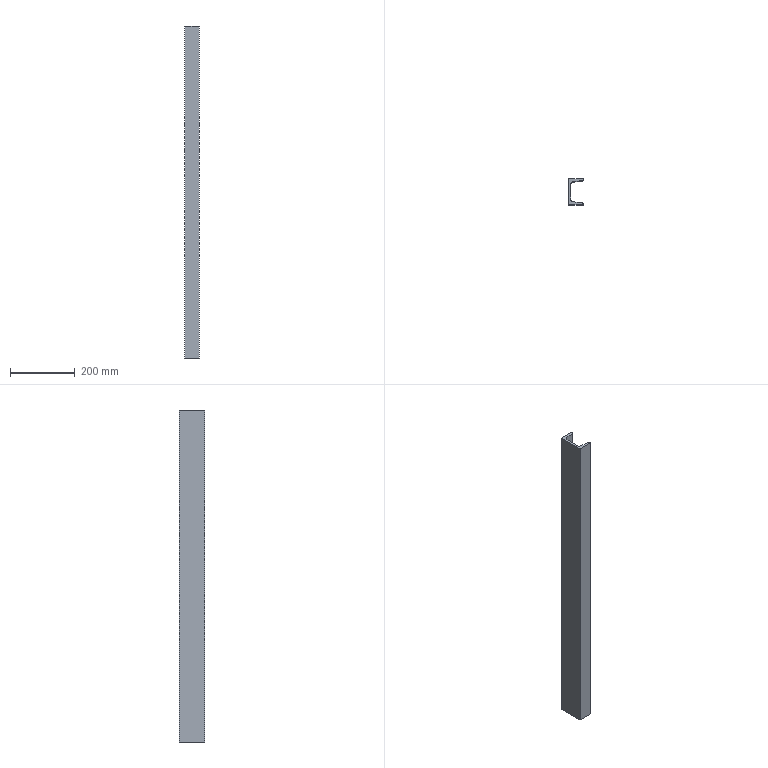Part | SolidWorks | features Extrusion 1 | 1 solid | 14 faces | box 45 x 80 x 1022 mm | volume 1109758 mm3 | plane 10 | cylinder 4 | commonest cylinder face diameters 8 x2 16 x2
STEP:
#1=CARTESIAN_POINT('',(-3.443,-5.322,0.));
#2=VERTEX_POINT('',#1);
#3=CARTESIAN_POINT('',(0.,-1.361,0.));
#4=VERTEX_POINT('',#3);
#5=CARTESIAN_POINT('',(-4.,-1.361,0.));
#6=DIRECTION('',(0.,0.,1.));
#7=DIRECTION('',(1.,0.,0.));
#8=AXIS2_PLACEMENT_3D('',#5,#6,#7);
#9=CIRCLE('',#8,4.);
#10=EDGE_CURVE('',#2,#4,#9,.T.);
#11=ORIENTED_EDGE('',*,*,#10,.T.);
#12=CARTESIAN_POINT('',(0.,-1.361,1022.));
#13=VERTEX_POINT('',#12);
#14=CARTESIAN_POINT('',(0.,-1.361,1022.));
#15=DIRECTION('',(0.,0.,-1.));
#16=VECTOR('',#15,1000.);
#17=LINE('',#14,#16);
#18=EDGE_CURVE('',#13,#4,#17,.T.);
#19=ORIENTED_EDGE('',*,*,#18,.F.);
#20=CARTESIAN_POINT('',(-3.443,-5.322,1022.));
#21=VERTEX_POINT('',#20);
#22=CARTESIAN_POINT('',(-4.,-1.361,1022.));
#23=DIRECTION('',(0.,0.,1.));
#24=DIRECTION('',(1.,0.,0.));
#25=AXIS2_PLACEMENT_3D('',#22,#23,#24);
#26=CIRCLE('',#25,4.);
#27=EDGE_CURVE('',#21,#13,#26,.T.);
#28=ORIENTED_EDGE('',*,*,#27,.F.);
#29=CARTESIAN_POINT('',(-3.443,-5.322,1022.));
#30=DIRECTION('',(0.,0.,-1.));
#31=VECTOR('',#30,1000.);
#32=LINE('',#29,#31);
#33=EDGE_CURVE('',#21,#2,#32,.T.);
#34=ORIENTED_EDGE('',*,*,#33,.T.);
#35=EDGE_LOOP('',(#11,#19,#28,#34));
#36=FACE_OUTER_BOUND('',#35,.T.);
#37=CARTESIAN_POINT('',(-4.,-1.361,1022.));
#38=DIRECTION('',(0.,0.,-1.));
#39=DIRECTION('',(-1.,0.,0.));
#40=AXIS2_PLACEMENT_3D('',#37,#38,#39);
#41=CYLINDRICAL_SURFACE('',#40,4.);
#42=ADVANCED_FACE('',(#36),#41,.T.);
#43=CARTESIAN_POINT('',(0.,0.,0.));
#44=VERTEX_POINT('',#43);
#45=CARTESIAN_POINT('',(0.,-1.361,0.));
#46=DIRECTION('',(0.,1.,0.));
#47=VECTOR('',#46,1000.);
#48=LINE('',#45,#47);
#49=EDGE_CURVE('',#4,#44,#48,.T.);
#50=ORIENTED_EDGE('',*,*,#49,.T.);
#51=CARTESIAN_POINT('',(0.,0.,1022.));
#52=VERTEX_POINT('',#51);
#53=CARTESIAN_POINT('',(0.,0.,1022.));
#54=DIRECTION('',(0.,0.,-1.));
#55=VECTOR('',#54,1000.);
#56=LINE('',#53,#55);
#57=EDGE_CURVE('',#52,#44,#56,.T.);
#58=ORIENTED_EDGE('',*,*,#57,.F.);
#59=CARTESIAN_POINT('',(0.,-1.361,1022.));
#60=DIRECTION('',(0.,1.,0.));
#61=VECTOR('',#60,1000.);
#62=LINE('',#59,#61);
#63=EDGE_CURVE('',#13,#52,#62,.T.);
#64=ORIENTED_EDGE('',*,*,#63,.F.);
#65=ORIENTED_EDGE('',*,*,#18,.T.);
#66=EDGE_LOOP('',(#50,#58,#64,#65));
#67=FACE_OUTER_BOUND('',#66,.T.);
#68=CARTESIAN_POINT('',(0.,-1.361,1022.));
#69=DIRECTION('',(-1.,0.,0.));
#70=DIRECTION('',(0.,0.,1.));
#71=AXIS2_PLACEMENT_3D('',#68,#69,#70);
#72=PLANE('',#71);
#73=ADVANCED_FACE('',(#67),#72,.F.);
#74=CARTESIAN_POINT('',(-45.,0.,0.));
#75=VERTEX_POINT('',#74);
#76=CARTESIAN_POINT('',(0.,0.,0.));
#77=DIRECTION('',(-1.,0.,0.));
#78=VECTOR('',#77,1000.);
#79=LINE('',#76,#78);
#80=EDGE_CURVE('',#44,#75,#79,.T.);
#81=ORIENTED_EDGE('',*,*,#80,.T.);
#82=CARTESIAN_POINT('',(-45.,0.,1022.));
#83=VERTEX_POINT('',#82);
#84=CARTESIAN_POINT('',(-45.,0.,1022.));
#85=DIRECTION('',(0.,0.,-1.));
#86=VECTOR('',#85,1000.);
#87=LINE('',#84,#86);
#88=EDGE_CURVE('',#83,#75,#87,.T.);
#89=ORIENTED_EDGE('',*,*,#88,.F.);
#90=CARTESIAN_POINT('',(0.,0.,1022.));
#91=DIRECTION('',(-1.,0.,0.));
#92=VECTOR('',#91,1000.);
#93=LINE('',#90,#92);
#94=EDGE_CURVE('',#52,#83,#93,.T.);
#95=ORIENTED_EDGE('',*,*,#94,.F.);
#96=ORIENTED_EDGE('',*,*,#57,.T.);
#97=EDGE_LOOP('',(#81,#89,#95,#96));
#98=FACE_OUTER_BOUND('',#97,.T.);
#99=CARTESIAN_POINT('',(0.,0.,1022.));
#100=DIRECTION('',(0.,-1.,0.));
#101=DIRECTION('',(1.,0.,0.));
#102=AXIS2_PLACEMENT_3D('',#99,#100,#101);
#103=PLANE('',#102);
#104=ADVANCED_FACE('',(#98),#103,.F.);
#105=CARTESIAN_POINT('',(-45.,-80.,0.));
#106=VERTEX_POINT('',#105);
#107=CARTESIAN_POINT('',(-45.,0.,0.));
#108=DIRECTION('',(0.,-1.,0.));
#109=VECTOR('',#108,1000.);
#110=LINE('',#107,#109);
#111=EDGE_CURVE('',#75,#106,#110,.T.);
#112=ORIENTED_EDGE('',*,*,#111,.T.);
#113=CARTESIAN_POINT('',(-45.,-80.,1022.));
#114=VERTEX_POINT('',#113);
#115=CARTESIAN_POINT('',(-45.,-80.,1022.));
#116=DIRECTION('',(0.,0.,-1.));
#117=VECTOR('',#116,1000.);
#118=LINE('',#115,#117);
#119=EDGE_CURVE('',#114,#106,#118,.T.);
#120=ORIENTED_EDGE('',*,*,#119,.F.);
#121=CARTESIAN_POINT('',(-45.,0.,1022.));
#122=DIRECTION('',(0.,-1.,0.));
#123=VECTOR('',#122,1000.);
#124=LINE('',#121,#123);
#125=EDGE_CURVE('',#83,#114,#124,.T.);
#126=ORIENTED_EDGE('',*,*,#125,.F.);
#127=ORIENTED_EDGE('',*,*,#88,.T.);
#128=EDGE_LOOP('',(#112,#120,#126,#127));
#129=FACE_OUTER_BOUND('',#128,.T.);
#130=CARTESIAN_POINT('',(-45.,0.,1022.));
#131=DIRECTION('',(1.,0.,0.));
#132=DIRECTION('',(0.,1.,0.));
#133=AXIS2_PLACEMENT_3D('',#130,#131,#132);
#134=PLANE('',#133);
#135=ADVANCED_FACE('',(#129),#134,.F.);
#136=CARTESIAN_POINT('',(0.,-80.,0.));
#137=VERTEX_POINT('',#136);
#138=CARTESIAN_POINT('',(-45.,-80.,0.));
#139=DIRECTION('',(1.,0.,0.));
#140=VECTOR('',#139,1000.);
#141=LINE('',#138,#140);
#142=EDGE_CURVE('',#106,#137,#141,.T.);
#143=ORIENTED_EDGE('',*,*,#142,.T.);
#144=CARTESIAN_POINT('',(0.,-80.,1022.));
#145=VERTEX_POINT('',#144);
#146=CARTESIAN_POINT('',(0.,-80.,1022.));
#147=DIRECTION('',(0.,0.,-1.));
#148=VECTOR('',#147,1000.);
#149=LINE('',#146,#148);
#150=EDGE_CURVE('',#145,#137,#149,.T.);
#151=ORIENTED_EDGE('',*,*,#150,.F.);
#152=CARTESIAN_POINT('',(-45.,-80.,1022.));
#153=DIRECTION('',(1.,0.,0.));
#154=VECTOR('',#153,1000.);
#155=LINE('',#152,#154);
#156=EDGE_CURVE('',#114,#145,#155,.T.);
#157=ORIENTED_EDGE('',*,*,#156,.F.);
#158=ORIENTED_EDGE('',*,*,#119,.T.);
#159=EDGE_LOOP('',(#143,#151,#157,#158));
#160=FACE_OUTER_BOUND('',#159,.T.);
#161=CARTESIAN_POINT('',(-45.,-80.,1022.));
#162=DIRECTION('',(0.,1.,0.));
#163=DIRECTION('',(-1.,0.,0.));
#164=AXIS2_PLACEMENT_3D('',#161,#162,#163);
#165=PLANE('',#164);
#166=ADVANCED_FACE('',(#160),#165,.F.);
#167=CARTESIAN_POINT('',(0.,-78.639,0.));
#168=VERTEX_POINT('',#167);
#169=CARTESIAN_POINT('',(0.,-80.,0.));
#170=DIRECTION('',(0.,1.,0.));
#171=VECTOR('',#170,1000.);
#172=LINE('',#169,#171);
#173=EDGE_CURVE('',#137,#168,#172,.T.);
#174=ORIENTED_EDGE('',*,*,#173,.T.);
#175=CARTESIAN_POINT('',(0.,-78.639,1022.));
#176=VERTEX_POINT('',#175);
#177=CARTESIAN_POINT('',(0.,-78.639,1022.));
#178=DIRECTION('',(0.,0.,-1.));
#179=VECTOR('',#178,1000.);
#180=LINE('',#177,#179);
#181=EDGE_CURVE('',#176,#168,#180,.T.);
#182=ORIENTED_EDGE('',*,*,#181,.F.);
#183=CARTESIAN_POINT('',(0.,-80.,1022.));
#184=DIRECTION('',(0.,1.,0.));
#185=VECTOR('',#184,1000.);
#186=LINE('',#183,#185);
#187=EDGE_CURVE('',#145,#176,#186,.T.);
#188=ORIENTED_EDGE('',*,*,#187,.F.);
#189=ORIENTED_EDGE('',*,*,#150,.T.);
#190=EDGE_LOOP('',(#174,#182,#188,#189));
#191=FACE_OUTER_BOUND('',#190,.T.);
#192=CARTESIAN_POINT('',(0.,-80.,1022.));
#193=DIRECTION('',(-1.,0.,0.));
#194=DIRECTION('',(0.,0.,1.));
#195=AXIS2_PLACEMENT_3D('',#192,#193,#194);
#196=PLANE('',#195);
#197=ADVANCED_FACE('',(#191),#196,.F.);
#198=CARTESIAN_POINT('',(-3.443,-74.678,0.));
#199=VERTEX_POINT('',#198);
#200=CARTESIAN_POINT('',(-4.,-78.639,0.));
#201=DIRECTION('',(0.,0.,1.));
#202=DIRECTION('',(1.,0.,0.));
#203=AXIS2_PLACEMENT_3D('',#200,#201,#202);
#204=CIRCLE('',#203,4.);
#205=EDGE_CURVE('',#168,#199,#204,.T.);
#206=ORIENTED_EDGE('',*,*,#205,.T.);
#207=CARTESIAN_POINT('',(-3.443,-74.678,1022.));
#208=VERTEX_POINT('',#207);
#209=CARTESIAN_POINT('',(-3.443,-74.678,1022.));
#210=DIRECTION('',(0.,0.,-1.));
#211=VECTOR('',#210,1000.);
#212=LINE('',#209,#211);
#213=EDGE_CURVE('',#208,#199,#212,.T.);
#214=ORIENTED_EDGE('',*,*,#213,.F.);
#215=CARTESIAN_POINT('',(-4.,-78.639,1022.));
#216=DIRECTION('',(0.,0.,1.));
#217=DIRECTION('',(1.,0.,0.));
#218=AXIS2_PLACEMENT_3D('',#215,#216,#217);
#219=CIRCLE('',#218,4.);
#220=EDGE_CURVE('',#176,#208,#219,.T.);
#221=ORIENTED_EDGE('',*,*,#220,.F.);
#222=ORIENTED_EDGE('',*,*,#181,.T.);
#223=EDGE_LOOP('',(#206,#214,#221,#222));
#224=FACE_OUTER_BOUND('',#223,.T.);
#225=CARTESIAN_POINT('',(-4.,-78.639,1022.));
#226=DIRECTION('',(0.,0.,-1.));
#227=DIRECTION('',(-1.,0.,0.));
#228=AXIS2_PLACEMENT_3D('',#225,#226,#227);
#229=CYLINDRICAL_SURFACE('',#228,4.);
#230=ADVANCED_FACE('',(#224),#229,.T.);
#231=CARTESIAN_POINT('',(-32.113,-70.649,0.));
#232=VERTEX_POINT('',#231);
#233=CARTESIAN_POINT('',(-3.443,-74.678,0.));
#234=DIRECTION('',(-0.9903,0.1392,0.));
#235=VECTOR('',#234,1000.);
#236=LINE('',#233,#235);
#237=EDGE_CURVE('',#199,#232,#236,.T.);
#238=ORIENTED_EDGE('',*,*,#237,.T.);
#239=CARTESIAN_POINT('',(-32.113,-70.649,1022.));
#240=VERTEX_POINT('',#239);
#241=CARTESIAN_POINT('',(-32.113,-70.649,1022.));
#242=DIRECTION('',(0.,0.,-1.));
#243=VECTOR('',#242,1000.);
#244=LINE('',#241,#243);
#245=EDGE_CURVE('',#240,#232,#244,.T.);
#246=ORIENTED_EDGE('',*,*,#245,.F.);
#247=CARTESIAN_POINT('',(-3.443,-74.678,1022.));
#248=DIRECTION('',(-0.9903,0.1392,0.));
#249=VECTOR('',#248,1000.);
#250=LINE('',#247,#249);
#251=EDGE_CURVE('',#208,#240,#250,.T.);
#252=ORIENTED_EDGE('',*,*,#251,.F.);
#253=ORIENTED_EDGE('',*,*,#213,.T.);
#254=EDGE_LOOP('',(#238,#246,#252,#253));
#255=FACE_OUTER_BOUND('',#254,.T.);
#256=CARTESIAN_POINT('',(-3.443,-74.678,1022.));
#257=DIRECTION('',(-0.1392,-0.9903,0.));
#258=DIRECTION('',(0.9903,-0.1392,0.));
#259=AXIS2_PLACEMENT_3D('',#256,#257,#258);
#260=PLANE('',#259);
#261=ADVANCED_FACE('',(#255),#260,.F.);
#262=CARTESIAN_POINT('',(-39.,-62.727,0.));
#263=VERTEX_POINT('',#262);
#264=CARTESIAN_POINT('',(-31.,-62.727,0.));
#265=DIRECTION('',(0.,0.,-1.));
#266=DIRECTION('',(-1.,0.,0.));
#267=AXIS2_PLACEMENT_3D('',#264,#265,#266);
#268=CIRCLE('',#267,8.);
#269=EDGE_CURVE('',#232,#263,#268,.T.);
#270=ORIENTED_EDGE('',*,*,#269,.T.);
#271=CARTESIAN_POINT('',(-39.,-62.727,1022.));
#272=VERTEX_POINT('',#271);
#273=CARTESIAN_POINT('',(-39.,-62.727,1022.));
#274=DIRECTION('',(0.,0.,-1.));
#275=VECTOR('',#274,1000.);
#276=LINE('',#273,#275);
#277=EDGE_CURVE('',#272,#263,#276,.T.);
#278=ORIENTED_EDGE('',*,*,#277,.F.);
#279=CARTESIAN_POINT('',(-31.,-62.727,1022.));
#280=DIRECTION('',(0.,0.,-1.));
#281=DIRECTION('',(-1.,0.,0.));
#282=AXIS2_PLACEMENT_3D('',#279,#280,#281);
#283=CIRCLE('',#282,8.);
#284=EDGE_CURVE('',#240,#272,#283,.T.);
#285=ORIENTED_EDGE('',*,*,#284,.F.);
#286=ORIENTED_EDGE('',*,*,#245,.T.);
#287=EDGE_LOOP('',(#270,#278,#285,#286));
#288=FACE_OUTER_BOUND('',#287,.T.);
#289=CARTESIAN_POINT('',(-31.,-62.727,1022.));
#290=DIRECTION('',(0.,0.,-1.));
#291=DIRECTION('',(-1.,0.,0.));
#292=AXIS2_PLACEMENT_3D('',#289,#290,#291);
#293=CYLINDRICAL_SURFACE('',#292,8.);
#294=ADVANCED_FACE('',(#288),#293,.F.);
#295=CARTESIAN_POINT('',(-39.,-17.273,0.));
#296=VERTEX_POINT('',#295);
#297=CARTESIAN_POINT('',(-39.,-62.727,0.));
#298=DIRECTION('',(0.,1.,0.));
#299=VECTOR('',#298,1000.);
#300=LINE('',#297,#299);
#301=EDGE_CURVE('',#263,#296,#300,.T.);
#302=ORIENTED_EDGE('',*,*,#301,.T.);
#303=CARTESIAN_POINT('',(-39.,-17.273,1022.));
#304=VERTEX_POINT('',#303);
#305=CARTESIAN_POINT('',(-39.,-17.273,1022.));
#306=DIRECTION('',(0.,0.,-1.));
#307=VECTOR('',#306,1000.);
#308=LINE('',#305,#307);
#309=EDGE_CURVE('',#304,#296,#308,.T.);
#310=ORIENTED_EDGE('',*,*,#309,.F.);
#311=CARTESIAN_POINT('',(-39.,-62.727,1022.));
#312=DIRECTION('',(0.,1.,0.));
#313=VECTOR('',#312,1000.);
#314=LINE('',#311,#313);
#315=EDGE_CURVE('',#272,#304,#314,.T.);
#316=ORIENTED_EDGE('',*,*,#315,.F.);
#317=ORIENTED_EDGE('',*,*,#277,.T.);
#318=EDGE_LOOP('',(#302,#310,#316,#317));
#319=FACE_OUTER_BOUND('',#318,.T.);
#320=CARTESIAN_POINT('',(-39.,-62.727,1022.));
#321=DIRECTION('',(-1.,0.,0.));
#322=DIRECTION('',(0.,0.,1.));
#323=AXIS2_PLACEMENT_3D('',#320,#321,#322);
#324=PLANE('',#323);
#325=ADVANCED_FACE('',(#319),#324,.F.);
#326=CARTESIAN_POINT('',(-32.113,-9.351,0.));
#327=VERTEX_POINT('',#326);
#328=CARTESIAN_POINT('',(-31.,-17.273,0.));
#329=DIRECTION('',(0.,0.,-1.));
#330=DIRECTION('',(-1.,0.,0.));
#331=AXIS2_PLACEMENT_3D('',#328,#329,#330);
#332=CIRCLE('',#331,8.);
#333=EDGE_CURVE('',#296,#327,#332,.T.);
#334=ORIENTED_EDGE('',*,*,#333,.T.);
#335=CARTESIAN_POINT('',(-32.113,-9.351,1022.));
#336=VERTEX_POINT('',#335);
#337=CARTESIAN_POINT('',(-32.113,-9.351,1022.));
#338=DIRECTION('',(0.,0.,-1.));
#339=VECTOR('',#338,1000.);
#340=LINE('',#337,#339);
#341=EDGE_CURVE('',#336,#327,#340,.T.);
#342=ORIENTED_EDGE('',*,*,#341,.F.);
#343=CARTESIAN_POINT('',(-31.,-17.273,1022.));
#344=DIRECTION('',(0.,0.,-1.));
#345=DIRECTION('',(-1.,0.,0.));
#346=AXIS2_PLACEMENT_3D('',#343,#344,#345);
#347=CIRCLE('',#346,8.);
#348=EDGE_CURVE('',#304,#336,#347,.T.);
#349=ORIENTED_EDGE('',*,*,#348,.F.);
#350=ORIENTED_EDGE('',*,*,#309,.T.);
#351=EDGE_LOOP('',(#334,#342,#349,#350));
#352=FACE_OUTER_BOUND('',#351,.T.);
#353=CARTESIAN_POINT('',(-31.,-17.273,1022.));
#354=DIRECTION('',(0.,0.,-1.));
#355=DIRECTION('',(-1.,0.,0.));
#356=AXIS2_PLACEMENT_3D('',#353,#354,#355);
#357=CYLINDRICAL_SURFACE('',#356,8.);
#358=ADVANCED_FACE('',(#352),#357,.F.);
#359=CARTESIAN_POINT('',(-32.113,-9.351,0.));
#360=DIRECTION('',(0.9903,0.1392,0.));
#361=VECTOR('',#360,1000.);
#362=LINE('',#359,#361);
#363=EDGE_CURVE('',#327,#2,#362,.T.);
#364=ORIENTED_EDGE('',*,*,#363,.T.);
#365=ORIENTED_EDGE('',*,*,#33,.F.);
#366=CARTESIAN_POINT('',(-32.113,-9.351,1022.));
#367=DIRECTION('',(0.9903,0.1392,0.));
#368=VECTOR('',#367,1000.);
#369=LINE('',#366,#368);
#370=EDGE_CURVE('',#336,#21,#369,.T.);
#371=ORIENTED_EDGE('',*,*,#370,.F.);
#372=ORIENTED_EDGE('',*,*,#341,.T.);
#373=EDGE_LOOP('',(#364,#365,#371,#372));
#374=FACE_OUTER_BOUND('',#373,.T.);
#375=CARTESIAN_POINT('',(-32.113,-9.351,1022.));
#376=DIRECTION('',(-0.1392,0.9903,0.));
#377=DIRECTION('',(-0.9903,-0.1392,0.));
#378=AXIS2_PLACEMENT_3D('',#375,#376,#377);
#379=PLANE('',#378);
#380=ADVANCED_FACE('',(#374),#379,.F.);
#381=ORIENTED_EDGE('',*,*,#27,.T.);
#382=ORIENTED_EDGE('',*,*,#63,.T.);
#383=ORIENTED_EDGE('',*,*,#94,.T.);
#384=ORIENTED_EDGE('',*,*,#125,.T.);
#385=ORIENTED_EDGE('',*,*,#156,.T.);
#386=ORIENTED_EDGE('',*,*,#187,.T.);
#387=ORIENTED_EDGE('',*,*,#220,.T.);
#388=ORIENTED_EDGE('',*,*,#251,.T.);
#389=ORIENTED_EDGE('',*,*,#284,.T.);
#390=ORIENTED_EDGE('',*,*,#315,.T.);
#391=ORIENTED_EDGE('',*,*,#348,.T.);
#392=ORIENTED_EDGE('',*,*,#370,.T.);
#393=EDGE_LOOP('',(#381,#382,#383,#384,#385,#386,#387,#388,#389,#390,#391,#392));
#394=FACE_OUTER_BOUND('',#393,.T.);
#395=CARTESIAN_POINT('',(-4.,-1.361,1022.));
#396=DIRECTION('',(0.,0.,1.));
#397=DIRECTION('',(1.,0.,0.));
#398=AXIS2_PLACEMENT_3D('',#395,#396,#397);
#399=PLANE('',#398);
#400=ADVANCED_FACE('',(#394),#399,.T.);
#401=ORIENTED_EDGE('',*,*,#10,.F.);
#402=ORIENTED_EDGE('',*,*,#363,.F.);
#403=ORIENTED_EDGE('',*,*,#333,.F.);
#404=ORIENTED_EDGE('',*,*,#301,.F.);
#405=ORIENTED_EDGE('',*,*,#269,.F.);
#406=ORIENTED_EDGE('',*,*,#237,.F.);
#407=ORIENTED_EDGE('',*,*,#205,.F.);
#408=ORIENTED_EDGE('',*,*,#173,.F.);
#409=ORIENTED_EDGE('',*,*,#142,.F.);
#410=ORIENTED_EDGE('',*,*,#111,.F.);
#411=ORIENTED_EDGE('',*,*,#80,.F.);
#412=ORIENTED_EDGE('',*,*,#49,.F.);
#413=EDGE_LOOP('',(#401,#402,#403,#404,#405,#406,#407,#408,#409,#410,#411,#412));
#414=FACE_OUTER_BOUND('',#413,.T.);
#415=CARTESIAN_POINT('',(-4.,-1.361,0.));
#416=DIRECTION('',(0.,0.,1.));
#417=DIRECTION('',(1.,0.,0.));
#418=AXIS2_PLACEMENT_3D('',#415,#416,#417);
#419=PLANE('',#418);
#420=ADVANCED_FACE('',(#414),#419,.F.);
#421=CLOSED_SHELL('',(#42,#73,#104,#135,#166,#197,#230,#261,#294,#325,#358,#380,#400,#420));
#422=MANIFOLD_SOLID_BREP('',#421);
#423=CARTESIAN_POINT('',(0.,0.,0.));
#424=DIRECTION('',(0.,0.,1.));
#425=DIRECTION('',(1.,0.,0.));
#426=AXIS2_PLACEMENT_3D('',#423,#424,#425);
#427=(LENGTH_UNIT()NAMED_UNIT(*)SI_UNIT(.MILLI.,.METRE.));
#428=UNCERTAINTY_MEASURE_WITH_UNIT(LENGTH_MEASURE(0.00001),#427,'','');
#429=(NAMED_UNIT(*)PLANE_ANGLE_UNIT()SI_UNIT($,.RADIAN.));
#430=(NAMED_UNIT(*)SI_UNIT($,.STERADIAN.)SOLID_ANGLE_UNIT());
#431=(GEOMETRIC_REPRESENTATION_CONTEXT(3)GLOBAL_UNCERTAINTY_ASSIGNED_CONTEXT((#428))GLOBAL_UNIT_ASSIGNED_CONTEXT((#427,#429,#430))REPRESENTATION_CONTEXT('',''));
#432=ADVANCED_BREP_SHAPE_REPRESENTATION('',(#422,#426),#431);